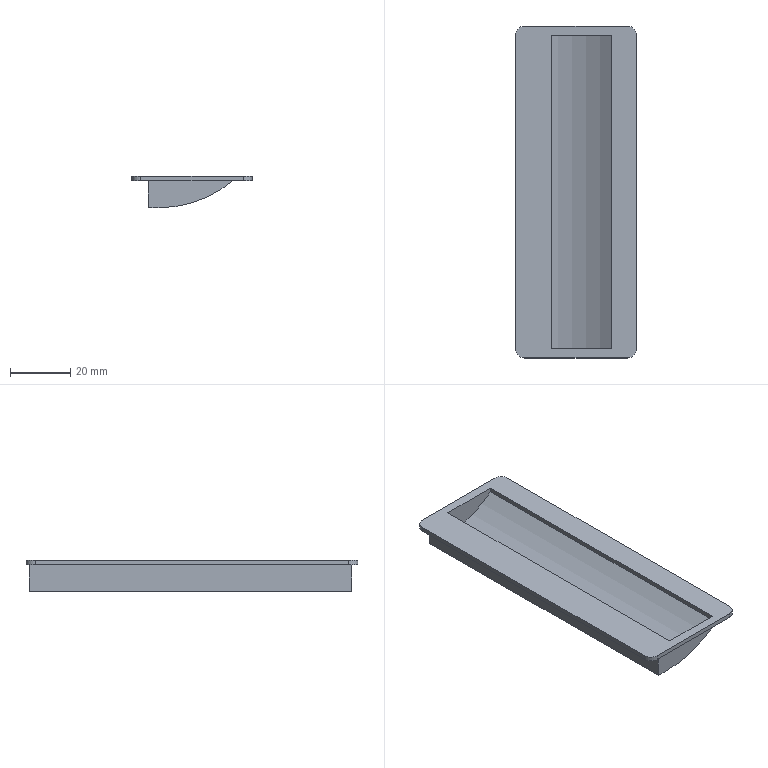Part | SolidWorks | features ICE 3, Extrusion 1, Fillet 1, MirrorPattern 1 | 1 solid | 23 faces | box 40 x 110 x 10.429 mm | volume 7857 mm3 | plane 15 | cylinder 8 | commonest cylinder face diameters 6 x4 73.801 x2 75.801 x2
STEP:
#1=CARTESIAN_POINT('',(-10.931,54.,-8.929));
#2=VERTEX_POINT('',#1);
#3=CARTESIAN_POINT('',(-14.495,54.,-8.761));
#4=VERTEX_POINT('',#3);
#5=CARTESIAN_POINT('',(-10.931,54.,28.971));
#6=DIRECTION('',(0.,1.,0.));
#7=DIRECTION('',(0.,0.,1.));
#8=AXIS2_PLACEMENT_3D('',#5,#6,#7);
#9=CIRCLE('',#8,37.9);
#10=EDGE_CURVE('',#2,#4,#9,.T.);
#11=ORIENTED_EDGE('',*,*,#10,.F.);
#12=CARTESIAN_POINT('',(-10.931,-53.,-8.929));
#13=VERTEX_POINT('',#12);
#14=CARTESIAN_POINT('',(-10.931,52.5,-8.929));
#15=DIRECTION('',(0.,-1.,0.));
#16=VECTOR('',#15,1000.);
#17=LINE('',#14,#16);
#18=EDGE_CURVE('',#2,#13,#17,.T.);
#19=ORIENTED_EDGE('',*,*,#18,.T.);
#20=CARTESIAN_POINT('',(-14.495,-53.,-8.761));
#21=VERTEX_POINT('',#20);
#22=CARTESIAN_POINT('',(-10.931,-53.,28.971));
#23=DIRECTION('',(0.,1.,0.));
#24=DIRECTION('',(0.,0.,1.));
#25=AXIS2_PLACEMENT_3D('',#22,#23,#24);
#26=CIRCLE('',#25,37.9);
#27=EDGE_CURVE('',#13,#21,#26,.T.);
#28=ORIENTED_EDGE('',*,*,#27,.T.);
#29=CARTESIAN_POINT('',(-14.495,52.5,-8.761));
#30=DIRECTION('',(0.,-1.,0.));
#31=VECTOR('',#30,1000.);
#32=LINE('',#29,#31);
#33=EDGE_CURVE('',#4,#21,#32,.T.);
#34=ORIENTED_EDGE('',*,*,#33,.F.);
#35=EDGE_LOOP('',(#11,#19,#28,#34));
#36=FACE_OUTER_BOUND('',#35,.T.);
#37=CARTESIAN_POINT('',(-10.931,52.5,28.971));
#38=DIRECTION('',(0.,-1.,0.));
#39=DIRECTION('',(0.,0.,-1.));
#40=AXIS2_PLACEMENT_3D('',#37,#38,#39);
#41=CYLINDRICAL_SURFACE('',#40,37.9);
#42=ADVANCED_FACE('',(#36),#41,.T.);
#43=CARTESIAN_POINT('',(-10.931,52.,-7.929));
#44=VERTEX_POINT('',#43);
#45=CARTESIAN_POINT('',(11.923,52.,0.));
#46=VERTEX_POINT('',#45);
#47=CARTESIAN_POINT('',(-10.931,52.,28.971));
#48=DIRECTION('',(0.,-1.,0.));
#49=DIRECTION('',(0.,0.,1.));
#50=AXIS2_PLACEMENT_3D('',#47,#48,#49);
#51=CIRCLE('',#50,36.9);
#52=EDGE_CURVE('',#44,#46,#51,.T.);
#53=ORIENTED_EDGE('',*,*,#52,.F.);
#54=CARTESIAN_POINT('',(-10.931,-52.,-7.929));
#55=VERTEX_POINT('',#54);
#56=CARTESIAN_POINT('',(-10.931,52.5,-7.929));
#57=DIRECTION('',(0.,-1.,0.));
#58=VECTOR('',#57,1000.);
#59=LINE('',#56,#58);
#60=EDGE_CURVE('',#44,#55,#59,.T.);
#61=ORIENTED_EDGE('',*,*,#60,.T.);
#62=CARTESIAN_POINT('',(11.923,-52.,0.));
#63=VERTEX_POINT('',#62);
#64=CARTESIAN_POINT('',(-10.931,-52.,28.971));
#65=DIRECTION('',(0.,1.,0.));
#66=DIRECTION('',(0.,0.,-1.));
#67=AXIS2_PLACEMENT_3D('',#64,#65,#66);
#68=CIRCLE('',#67,36.9);
#69=EDGE_CURVE('',#63,#55,#68,.T.);
#70=ORIENTED_EDGE('',*,*,#69,.F.);
#71=CARTESIAN_POINT('',(11.923,52.5,0.));
#72=DIRECTION('',(0.,-1.,0.));
#73=VECTOR('',#72,1000.);
#74=LINE('',#71,#73);
#75=EDGE_CURVE('',#46,#63,#74,.T.);
#76=ORIENTED_EDGE('',*,*,#75,.F.);
#77=EDGE_LOOP('',(#53,#61,#70,#76));
#78=FACE_OUTER_BOUND('',#77,.T.);
#79=CARTESIAN_POINT('',(-10.931,52.5,28.971));
#80=DIRECTION('',(0.,-1.,0.));
#81=DIRECTION('',(0.,0.,-1.));
#82=AXIS2_PLACEMENT_3D('',#79,#80,#81);
#83=CYLINDRICAL_SURFACE('',#82,36.9);
#84=ADVANCED_FACE('',(#78),#83,.F.);
#85=ORIENTED_EDGE('',*,*,#69,.T.);
#86=CARTESIAN_POINT('',(-13.495,-52.,-7.84));
#87=VERTEX_POINT('',#86);
#88=CARTESIAN_POINT('',(-10.931,-52.,28.971));
#89=DIRECTION('',(0.,1.,0.));
#90=DIRECTION('',(0.,0.,-1.));
#91=AXIS2_PLACEMENT_3D('',#88,#89,#90);
#92=CIRCLE('',#91,36.9);
#93=EDGE_CURVE('',#55,#87,#92,.T.);
#94=ORIENTED_EDGE('',*,*,#93,.T.);
#95=CARTESIAN_POINT('',(-13.495,-52.,0.));
#96=VERTEX_POINT('',#95);
#97=CARTESIAN_POINT('',(-13.495,-52.,0.));
#98=DIRECTION('',(0.,0.,1.));
#99=VECTOR('',#98,1000.);
#100=LINE('',#97,#99);
#101=EDGE_CURVE('',#87,#96,#100,.T.);
#102=ORIENTED_EDGE('',*,*,#101,.T.);
#103=CARTESIAN_POINT('',(-8.077,-52.,0.));
#104=VERTEX_POINT('',#103);
#105=CARTESIAN_POINT('',(-14.495,-52.,0.));
#106=DIRECTION('',(1.,0.,0.));
#107=VECTOR('',#106,1000.);
#108=LINE('',#105,#107);
#109=EDGE_CURVE('',#96,#104,#108,.T.);
#110=ORIENTED_EDGE('',*,*,#109,.T.);
#111=CARTESIAN_POINT('',(-8.077,-52.,1.5));
#112=VERTEX_POINT('',#111);
#113=CARTESIAN_POINT('',(-8.077,-52.,0.));
#114=DIRECTION('',(0.,0.,1.));
#115=VECTOR('',#114,1000.);
#116=LINE('',#113,#115);
#117=EDGE_CURVE('',#104,#112,#116,.T.);
#118=ORIENTED_EDGE('',*,*,#117,.T.);
#119=CARTESIAN_POINT('',(11.923,-52.,1.5));
#120=VERTEX_POINT('',#119);
#121=CARTESIAN_POINT('',(-8.077,-52.,1.5));
#122=DIRECTION('',(1.,0.,0.));
#123=VECTOR('',#122,1000.);
#124=LINE('',#121,#123);
#125=EDGE_CURVE('',#112,#120,#124,.T.);
#126=ORIENTED_EDGE('',*,*,#125,.T.);
#127=CARTESIAN_POINT('',(11.923,-52.,0.));
#128=DIRECTION('',(0.,0.,1.));
#129=VECTOR('',#128,1000.);
#130=LINE('',#127,#129);
#131=EDGE_CURVE('',#63,#120,#130,.T.);
#132=ORIENTED_EDGE('',*,*,#131,.F.);
#133=EDGE_LOOP('',(#85,#94,#102,#110,#118,#126,#132));
#134=FACE_OUTER_BOUND('',#133,.T.);
#135=CARTESIAN_POINT('',(-10.931,-52.,28.971));
#136=DIRECTION('',(0.,-1.,0.));
#137=DIRECTION('',(0.,0.,1.));
#138=AXIS2_PLACEMENT_3D('',#135,#136,#137);
#139=PLANE('',#138);
#140=ADVANCED_FACE('',(#134),#139,.F.);
#141=CARTESIAN_POINT('',(-13.495,52.,0.));
#142=VERTEX_POINT('',#141);
#143=CARTESIAN_POINT('',(-8.077,52.,0.));
#144=VERTEX_POINT('',#143);
#145=CARTESIAN_POINT('',(11.923,52.,0.));
#146=DIRECTION('',(1.,0.,0.));
#147=VECTOR('',#146,1000.);
#148=LINE('',#145,#147);
#149=EDGE_CURVE('',#142,#144,#148,.T.);
#150=ORIENTED_EDGE('',*,*,#149,.F.);
#151=CARTESIAN_POINT('',(-13.495,52.,-7.84));
#152=VERTEX_POINT('',#151);
#153=CARTESIAN_POINT('',(-13.495,52.,0.));
#154=DIRECTION('',(0.,0.,-1.));
#155=VECTOR('',#154,1000.);
#156=LINE('',#153,#155);
#157=EDGE_CURVE('',#142,#152,#156,.T.);
#158=ORIENTED_EDGE('',*,*,#157,.T.);
#159=CARTESIAN_POINT('',(-10.931,52.,28.971));
#160=DIRECTION('',(0.,-1.,0.));
#161=DIRECTION('',(0.,0.,1.));
#162=AXIS2_PLACEMENT_3D('',#159,#160,#161);
#163=CIRCLE('',#162,36.9);
#164=EDGE_CURVE('',#152,#44,#163,.T.);
#165=ORIENTED_EDGE('',*,*,#164,.T.);
#166=ORIENTED_EDGE('',*,*,#52,.T.);
#167=CARTESIAN_POINT('',(11.923,52.,1.5));
#168=VERTEX_POINT('',#167);
#169=CARTESIAN_POINT('',(11.923,52.,0.));
#170=DIRECTION('',(0.,0.,1.));
#171=VECTOR('',#170,1000.);
#172=LINE('',#169,#171);
#173=EDGE_CURVE('',#46,#168,#172,.T.);
#174=ORIENTED_EDGE('',*,*,#173,.T.);
#175=CARTESIAN_POINT('',(-8.077,52.,1.5));
#176=VERTEX_POINT('',#175);
#177=CARTESIAN_POINT('',(-8.077,52.,1.5));
#178=DIRECTION('',(-1.,0.,0.));
#179=VECTOR('',#178,1000.);
#180=LINE('',#177,#179);
#181=EDGE_CURVE('',#168,#176,#180,.T.);
#182=ORIENTED_EDGE('',*,*,#181,.T.);
#183=CARTESIAN_POINT('',(-8.077,52.,0.));
#184=DIRECTION('',(0.,0.,1.));
#185=VECTOR('',#184,1000.);
#186=LINE('',#183,#185);
#187=EDGE_CURVE('',#144,#176,#186,.T.);
#188=ORIENTED_EDGE('',*,*,#187,.F.);
#189=EDGE_LOOP('',(#150,#158,#165,#166,#174,#182,#188));
#190=FACE_OUTER_BOUND('',#189,.T.);
#191=CARTESIAN_POINT('',(-10.931,52.,28.971));
#192=DIRECTION('',(0.,1.,0.));
#193=DIRECTION('',(0.,0.,1.));
#194=AXIS2_PLACEMENT_3D('',#191,#192,#193);
#195=PLANE('',#194);
#196=ADVANCED_FACE('',(#190),#195,.F.);
#197=ORIENTED_EDGE('',*,*,#60,.F.);
#198=ORIENTED_EDGE('',*,*,#164,.F.);
#199=CARTESIAN_POINT('',(-13.495,52.5,-7.84));
#200=DIRECTION('',(0.,-1.,0.));
#201=VECTOR('',#200,1000.);
#202=LINE('',#199,#201);
#203=EDGE_CURVE('',#152,#87,#202,.T.);
#204=ORIENTED_EDGE('',*,*,#203,.T.);
#205=ORIENTED_EDGE('',*,*,#93,.F.);
#206=EDGE_LOOP('',(#197,#198,#204,#205));
#207=FACE_OUTER_BOUND('',#206,.T.);
#208=CARTESIAN_POINT('',(-10.931,52.5,28.971));
#209=DIRECTION('',(0.,-1.,0.));
#210=DIRECTION('',(0.,0.,-1.));
#211=AXIS2_PLACEMENT_3D('',#208,#209,#210);
#212=CYLINDRICAL_SURFACE('',#211,36.9);
#213=ADVANCED_FACE('',(#207),#212,.F.);
#214=ORIENTED_EDGE('',*,*,#101,.F.);
#215=ORIENTED_EDGE('',*,*,#203,.F.);
#216=ORIENTED_EDGE('',*,*,#157,.F.);
#217=CARTESIAN_POINT('',(-13.495,52.5,0.));
#218=DIRECTION('',(0.,-1.,0.));
#219=VECTOR('',#218,1000.);
#220=LINE('',#217,#219);
#221=EDGE_CURVE('',#142,#96,#220,.T.);
#222=ORIENTED_EDGE('',*,*,#221,.T.);
#223=EDGE_LOOP('',(#214,#215,#216,#222));
#224=FACE_OUTER_BOUND('',#223,.T.);
#225=CARTESIAN_POINT('',(-13.495,52.5,0.));
#226=DIRECTION('',(-1.,0.,0.));
#227=DIRECTION('',(0.,0.,1.));
#228=AXIS2_PLACEMENT_3D('',#225,#226,#227);
#229=PLANE('',#228);
#230=ADVANCED_FACE('',(#224),#229,.F.);
#231=CARTESIAN_POINT('',(-8.077,-52.,0.));
#232=DIRECTION('',(0.,-1.,0.));
#233=VECTOR('',#232,1000.);
#234=LINE('',#231,#233);
#235=EDGE_CURVE('',#144,#104,#234,.T.);
#236=ORIENTED_EDGE('',*,*,#235,.T.);
#237=ORIENTED_EDGE('',*,*,#109,.F.);
#238=ORIENTED_EDGE('',*,*,#221,.F.);
#239=ORIENTED_EDGE('',*,*,#149,.T.);
#240=EDGE_LOOP('',(#236,#237,#238,#239));
#241=FACE_OUTER_BOUND('',#240,.T.);
#242=CARTESIAN_POINT('',(0.,0.,0.));
#243=DIRECTION('',(0.,0.,-1.));
#244=DIRECTION('',(-1.,0.,0.));
#245=AXIS2_PLACEMENT_3D('',#242,#243,#244);
#246=PLANE('',#245);
#247=ADVANCED_FACE('',(#241),#246,.T.);
#248=CARTESIAN_POINT('',(11.923,-52.,1.5));
#249=DIRECTION('',(0.,1.,0.));
#250=VECTOR('',#249,1000.);
#251=LINE('',#248,#250);
#252=EDGE_CURVE('',#120,#168,#251,.T.);
#253=ORIENTED_EDGE('',*,*,#252,.T.);
#254=ORIENTED_EDGE('',*,*,#173,.F.);
#255=ORIENTED_EDGE('',*,*,#75,.T.);
#256=ORIENTED_EDGE('',*,*,#131,.T.);
#257=EDGE_LOOP('',(#253,#254,#255,#256));
#258=FACE_OUTER_BOUND('',#257,.T.);
#259=CARTESIAN_POINT('',(11.923,-52.,0.));
#260=DIRECTION('',(1.,0.,0.));
#261=DIRECTION('',(0.,0.,-1.));
#262=AXIS2_PLACEMENT_3D('',#259,#260,#261);
#263=PLANE('',#262);
#264=ADVANCED_FACE('',(#258),#263,.F.);
#265=CARTESIAN_POINT('',(-8.077,-52.,1.5));
#266=DIRECTION('',(0.,-1.,0.));
#267=VECTOR('',#266,1000.);
#268=LINE('',#265,#267);
#269=EDGE_CURVE('',#176,#112,#268,.T.);
#270=ORIENTED_EDGE('',*,*,#269,.T.);
#271=ORIENTED_EDGE('',*,*,#117,.F.);
#272=ORIENTED_EDGE('',*,*,#235,.F.);
#273=ORIENTED_EDGE('',*,*,#187,.T.);
#274=EDGE_LOOP('',(#270,#271,#272,#273));
#275=FACE_OUTER_BOUND('',#274,.T.);
#276=CARTESIAN_POINT('',(-8.077,-52.,0.));
#277=DIRECTION('',(-1.,0.,0.));
#278=DIRECTION('',(0.,0.,1.));
#279=AXIS2_PLACEMENT_3D('',#276,#277,#278);
#280=PLANE('',#279);
#281=ADVANCED_FACE('',(#275),#280,.F.);
#282=CARTESIAN_POINT('',(-14.495,54.,0.));
#283=VERTEX_POINT('',#282);
#284=CARTESIAN_POINT('',(13.505,54.,0.));
#285=VERTEX_POINT('',#284);
#286=CARTESIAN_POINT('',(-14.495,54.,0.));
#287=DIRECTION('',(1.,0.,0.));
#288=VECTOR('',#287,1000.);
#289=LINE('',#286,#288);
#290=EDGE_CURVE('',#283,#285,#289,.T.);
#291=ORIENTED_EDGE('',*,*,#290,.F.);
#292=CARTESIAN_POINT('',(-14.495,-53.,0.));
#293=VERTEX_POINT('',#292);
#294=CARTESIAN_POINT('',(-14.495,52.5,0.));
#295=DIRECTION('',(0.,-1.,0.));
#296=VECTOR('',#295,1000.);
#297=LINE('',#294,#296);
#298=EDGE_CURVE('',#283,#293,#297,.T.);
#299=ORIENTED_EDGE('',*,*,#298,.T.);
#300=CARTESIAN_POINT('',(13.505,-53.,0.));
#301=VERTEX_POINT('',#300);
#302=CARTESIAN_POINT('',(11.923,-53.,0.));
#303=DIRECTION('',(1.,0.,0.));
#304=VECTOR('',#303,1000.);
#305=LINE('',#302,#304);
#306=EDGE_CURVE('',#293,#301,#305,.T.);
#307=ORIENTED_EDGE('',*,*,#306,.T.);
#308=CARTESIAN_POINT('',(13.505,52.5,0.));
#309=DIRECTION('',(0.,-1.,0.));
#310=VECTOR('',#309,1000.);
#311=LINE('',#308,#310);
#312=EDGE_CURVE('',#285,#301,#311,.T.);
#313=ORIENTED_EDGE('',*,*,#312,.F.);
#314=EDGE_LOOP('',(#291,#299,#307,#313));
#315=FACE_BOUND('',#314,.T.);
#316=CARTESIAN_POINT('',(20.,-52.,0.));
#317=VERTEX_POINT('',#316);
#318=CARTESIAN_POINT('',(20.,52.,0.));
#319=VERTEX_POINT('',#318);
#320=CARTESIAN_POINT('',(20.,-55.,0.));
#321=DIRECTION('',(0.,1.,0.));
#322=VECTOR('',#321,1000.);
#323=LINE('',#320,#322);
#324=EDGE_CURVE('',#317,#319,#323,.T.);
#325=ORIENTED_EDGE('',*,*,#324,.F.);
#326=CARTESIAN_POINT('',(17.,-55.,0.));
#327=VERTEX_POINT('',#326);
#328=CARTESIAN_POINT('',(17.,-52.,0.));
#329=DIRECTION('',(0.,0.,-1.));
#330=DIRECTION('',(-1.,0.,0.));
#331=AXIS2_PLACEMENT_3D('',#328,#329,#330);
#332=CIRCLE('',#331,3.);
#333=EDGE_CURVE('',#317,#327,#332,.T.);
#334=ORIENTED_EDGE('',*,*,#333,.T.);
#335=CARTESIAN_POINT('',(-17.,-55.,0.));
#336=VERTEX_POINT('',#335);
#337=CARTESIAN_POINT('',(-20.,-55.,0.));
#338=DIRECTION('',(1.,0.,0.));
#339=VECTOR('',#338,1000.);
#340=LINE('',#337,#339);
#341=EDGE_CURVE('',#336,#327,#340,.T.);
#342=ORIENTED_EDGE('',*,*,#341,.F.);
#343=CARTESIAN_POINT('',(-20.,-52.,0.));
#344=VERTEX_POINT('',#343);
#345=CARTESIAN_POINT('',(-17.,-52.,0.));
#346=DIRECTION('',(0.,0.,-1.));
#347=DIRECTION('',(-1.,0.,0.));
#348=AXIS2_PLACEMENT_3D('',#345,#346,#347);
#349=CIRCLE('',#348,3.);
#350=EDGE_CURVE('',#336,#344,#349,.T.);
#351=ORIENTED_EDGE('',*,*,#350,.T.);
#352=CARTESIAN_POINT('',(-20.,52.,0.));
#353=VERTEX_POINT('',#352);
#354=CARTESIAN_POINT('',(-20.,-55.,0.));
#355=DIRECTION('',(0.,-1.,0.));
#356=VECTOR('',#355,1000.);
#357=LINE('',#354,#356);
#358=EDGE_CURVE('',#353,#344,#357,.T.);
#359=ORIENTED_EDGE('',*,*,#358,.F.);
#360=CARTESIAN_POINT('',(-17.,55.,0.));
#361=VERTEX_POINT('',#360);
#362=CARTESIAN_POINT('',(-17.,52.,0.));
#363=DIRECTION('',(0.,0.,-1.));
#364=DIRECTION('',(-1.,0.,0.));
#365=AXIS2_PLACEMENT_3D('',#362,#363,#364);
#366=CIRCLE('',#365,3.);
#367=EDGE_CURVE('',#353,#361,#366,.T.);
#368=ORIENTED_EDGE('',*,*,#367,.T.);
#369=CARTESIAN_POINT('',(17.,55.,0.));
#370=VERTEX_POINT('',#369);
#371=CARTESIAN_POINT('',(-20.,55.,0.));
#372=DIRECTION('',(-1.,0.,0.));
#373=VECTOR('',#372,1000.);
#374=LINE('',#371,#373);
#375=EDGE_CURVE('',#370,#361,#374,.T.);
#376=ORIENTED_EDGE('',*,*,#375,.F.);
#377=CARTESIAN_POINT('',(17.,52.,0.));
#378=DIRECTION('',(0.,0.,-1.));
#379=DIRECTION('',(-1.,0.,0.));
#380=AXIS2_PLACEMENT_3D('',#377,#378,#379);
#381=CIRCLE('',#380,3.);
#382=EDGE_CURVE('',#370,#319,#381,.T.);
#383=ORIENTED_EDGE('',*,*,#382,.T.);
#384=EDGE_LOOP('',(#325,#334,#342,#351,#359,#368,#376,#383));
#385=FACE_OUTER_BOUND('',#384,.T.);
#386=CARTESIAN_POINT('',(0.,0.,0.));
#387=DIRECTION('',(0.,0.,-1.));
#388=DIRECTION('',(-1.,0.,0.));
#389=AXIS2_PLACEMENT_3D('',#386,#387,#388);
#390=PLANE('',#389);
#391=ADVANCED_FACE('',(#315,#385),#390,.T.);
#392=CARTESIAN_POINT('',(20.,-52.,1.5));
#393=VERTEX_POINT('',#392);
#394=CARTESIAN_POINT('',(20.,52.,1.5));
#395=VERTEX_POINT('',#394);
#396=CARTESIAN_POINT('',(20.,-55.,1.5));
#397=DIRECTION('',(0.,1.,0.));
#398=VECTOR('',#397,1000.);
#399=LINE('',#396,#398);
#400=EDGE_CURVE('',#393,#395,#399,.T.);
#401=ORIENTED_EDGE('',*,*,#400,.F.);
#402=CARTESIAN_POINT('',(20.,-52.,1.5));
#403=DIRECTION('',(0.,0.,-1.));
#404=VECTOR('',#403,1000.);
#405=LINE('',#402,#404);
#406=EDGE_CURVE('',#393,#317,#405,.T.);
#407=ORIENTED_EDGE('',*,*,#406,.T.);
#408=ORIENTED_EDGE('',*,*,#324,.T.);
#409=CARTESIAN_POINT('',(20.,52.,1.5));
#410=DIRECTION('',(0.,0.,1.));
#411=VECTOR('',#410,1000.);
#412=LINE('',#409,#411);
#413=EDGE_CURVE('',#319,#395,#412,.T.);
#414=ORIENTED_EDGE('',*,*,#413,.T.);
#415=EDGE_LOOP('',(#401,#407,#408,#414));
#416=FACE_OUTER_BOUND('',#415,.T.);
#417=CARTESIAN_POINT('',(20.,-55.,1.5));
#418=DIRECTION('',(-1.,0.,0.));
#419=DIRECTION('',(0.,0.,1.));
#420=AXIS2_PLACEMENT_3D('',#417,#418,#419);
#421=PLANE('',#420);
#422=ADVANCED_FACE('',(#416),#421,.F.);
#423=ORIENTED_EDGE('',*,*,#375,.T.);
#424=CARTESIAN_POINT('',(-17.,55.,1.5));
#425=VERTEX_POINT('',#424);
#426=CARTESIAN_POINT('',(-17.,55.,1.5));
#427=DIRECTION('',(0.,0.,1.));
#428=VECTOR('',#427,1000.);
#429=LINE('',#426,#428);
#430=EDGE_CURVE('',#361,#425,#429,.T.);
#431=ORIENTED_EDGE('',*,*,#430,.T.);
#432=CARTESIAN_POINT('',(17.,55.,1.5));
#433=VERTEX_POINT('',#432);
#434=CARTESIAN_POINT('',(-20.,55.,1.5));
#435=DIRECTION('',(-1.,0.,0.));
#436=VECTOR('',#435,1000.);
#437=LINE('',#434,#436);
#438=EDGE_CURVE('',#433,#425,#437,.T.);
#439=ORIENTED_EDGE('',*,*,#438,.F.);
#440=CARTESIAN_POINT('',(17.,55.,1.5));
#441=DIRECTION('',(0.,0.,-1.));
#442=VECTOR('',#441,1000.);
#443=LINE('',#440,#442);
#444=EDGE_CURVE('',#433,#370,#443,.T.);
#445=ORIENTED_EDGE('',*,*,#444,.T.);
#446=EDGE_LOOP('',(#423,#431,#439,#445));
#447=FACE_OUTER_BOUND('',#446,.T.);
#448=CARTESIAN_POINT('',(-20.,55.,1.5));
#449=DIRECTION('',(0.,-1.,0.));
#450=DIRECTION('',(0.,0.,-1.));
#451=AXIS2_PLACEMENT_3D('',#448,#449,#450);
#452=PLANE('',#451);
#453=ADVANCED_FACE('',(#447),#452,.F.);
#454=ORIENTED_EDGE('',*,*,#358,.T.);
#455=CARTESIAN_POINT('',(-20.,-52.,1.5));
#456=VERTEX_POINT('',#455);
#457=CARTESIAN_POINT('',(-20.,-52.,1.5));
#458=DIRECTION('',(0.,0.,1.));
#459=VECTOR('',#458,1000.);
#460=LINE('',#457,#459);
#461=EDGE_CURVE('',#344,#456,#460,.T.);
#462=ORIENTED_EDGE('',*,*,#461,.T.);
#463=CARTESIAN_POINT('',(-20.,52.,1.5));
#464=VERTEX_POINT('',#463);
#465=CARTESIAN_POINT('',(-20.,-55.,1.5));
#466=DIRECTION('',(0.,-1.,0.));
#467=VECTOR('',#466,1000.);
#468=LINE('',#465,#467);
#469=EDGE_CURVE('',#464,#456,#468,.T.);
#470=ORIENTED_EDGE('',*,*,#469,.F.);
#471=CARTESIAN_POINT('',(-20.,52.,1.5));
#472=DIRECTION('',(0.,0.,-1.));
#473=VECTOR('',#472,1000.);
#474=LINE('',#471,#473);
#475=EDGE_CURVE('',#464,#353,#474,.T.);
#476=ORIENTED_EDGE('',*,*,#475,.T.);
#477=EDGE_LOOP('',(#454,#462,#470,#476));
#478=FACE_OUTER_BOUND('',#477,.T.);
#479=CARTESIAN_POINT('',(-20.,-55.,1.5));
#480=DIRECTION('',(1.,0.,0.));
#481=DIRECTION('',(0.,0.,-1.));
#482=AXIS2_PLACEMENT_3D('',#479,#480,#481);
#483=PLANE('',#482);
#484=ADVANCED_FACE('',(#478),#483,.F.);
#485=ORIENTED_EDGE('',*,*,#341,.T.);
#486=CARTESIAN_POINT('',(17.,-55.,1.5));
#487=VERTEX_POINT('',#486);
#488=CARTESIAN_POINT('',(17.,-55.,1.5));
#489=DIRECTION('',(0.,0.,1.));
#490=VECTOR('',#489,1000.);
#491=LINE('',#488,#490);
#492=EDGE_CURVE('',#327,#487,#491,.T.);
#493=ORIENTED_EDGE('',*,*,#492,.T.);
#494=CARTESIAN_POINT('',(-17.,-55.,1.5));
#495=VERTEX_POINT('',#494);
#496=CARTESIAN_POINT('',(-20.,-55.,1.5));
#497=DIRECTION('',(1.,0.,0.));
#498=VECTOR('',#497,1000.);
#499=LINE('',#496,#498);
#500=EDGE_CURVE('',#495,#487,#499,.T.);
#501=ORIENTED_EDGE('',*,*,#500,.F.);
#502=CARTESIAN_POINT('',(-17.,-55.,1.5));
#503=DIRECTION('',(0.,0.,-1.));
#504=VECTOR('',#503,1000.);
#505=LINE('',#502,#504);
#506=EDGE_CURVE('',#495,#336,#505,.T.);
#507=ORIENTED_EDGE('',*,*,#506,.T.);
#508=EDGE_LOOP('',(#485,#493,#501,#507));
#509=FACE_OUTER_BOUND('',#508,.T.);
#510=CARTESIAN_POINT('',(-20.,-55.,1.5));
#511=DIRECTION('',(0.,1.,0.));
#512=DIRECTION('',(0.,0.,1.));
#513=AXIS2_PLACEMENT_3D('',#510,#511,#512);
#514=PLANE('',#513);
#515=ADVANCED_FACE('',(#509),#514,.F.);
#516=ORIENTED_EDGE('',*,*,#181,.F.);
#517=ORIENTED_EDGE('',*,*,#252,.F.);
#518=ORIENTED_EDGE('',*,*,#125,.F.);
#519=ORIENTED_EDGE('',*,*,#269,.F.);
#520=EDGE_LOOP('',(#516,#517,#518,#519));
#521=FACE_BOUND('',#520,.T.);
#522=ORIENTED_EDGE('',*,*,#500,.T.);
#523=CARTESIAN_POINT('',(17.,-52.,1.5));
#524=DIRECTION('',(0.,0.,1.));
#525=DIRECTION('',(-1.,0.,0.));
#526=AXIS2_PLACEMENT_3D('',#523,#524,#525);
#527=CIRCLE('',#526,3.);
#528=EDGE_CURVE('',#487,#393,#527,.T.);
#529=ORIENTED_EDGE('',*,*,#528,.T.);
#530=ORIENTED_EDGE('',*,*,#400,.T.);
#531=CARTESIAN_POINT('',(17.,52.,1.5));
#532=DIRECTION('',(0.,0.,1.));
#533=DIRECTION('',(-1.,0.,0.));
#534=AXIS2_PLACEMENT_3D('',#531,#532,#533);
#535=CIRCLE('',#534,3.);
#536=EDGE_CURVE('',#395,#433,#535,.T.);
#537=ORIENTED_EDGE('',*,*,#536,.T.);
#538=ORIENTED_EDGE('',*,*,#438,.T.);
#539=CARTESIAN_POINT('',(-17.,52.,1.5));
#540=DIRECTION('',(0.,0.,1.));
#541=DIRECTION('',(-1.,0.,0.));
#542=AXIS2_PLACEMENT_3D('',#539,#540,#541);
#543=CIRCLE('',#542,3.);
#544=EDGE_CURVE('',#425,#464,#543,.T.);
#545=ORIENTED_EDGE('',*,*,#544,.T.);
#546=ORIENTED_EDGE('',*,*,#469,.T.);
#547=CARTESIAN_POINT('',(-17.,-52.,1.5));
#548=DIRECTION('',(0.,0.,1.));
#549=DIRECTION('',(-1.,0.,0.));
#550=AXIS2_PLACEMENT_3D('',#547,#548,#549);
#551=CIRCLE('',#550,3.);
#552=EDGE_CURVE('',#456,#495,#551,.T.);
#553=ORIENTED_EDGE('',*,*,#552,.T.);
#554=EDGE_LOOP('',(#522,#529,#530,#537,#538,#545,#546,#553));
#555=FACE_OUTER_BOUND('',#554,.T.);
#556=CARTESIAN_POINT('',(0.,0.,1.5));
#557=DIRECTION('',(0.,0.,-1.));
#558=DIRECTION('',(-1.,0.,0.));
#559=AXIS2_PLACEMENT_3D('',#556,#557,#558);
#560=PLANE('',#559);
#561=ADVANCED_FACE('',(#521,#555),#560,.F.);
#562=ORIENTED_EDGE('',*,*,#18,.F.);
#563=CARTESIAN_POINT('',(-10.931,54.,28.971));
#564=DIRECTION('',(0.,1.,0.));
#565=DIRECTION('',(0.,0.,1.));
#566=AXIS2_PLACEMENT_3D('',#563,#564,#565);
#567=CIRCLE('',#566,37.9);
#568=EDGE_CURVE('',#285,#2,#567,.T.);
#569=ORIENTED_EDGE('',*,*,#568,.F.);
#570=ORIENTED_EDGE('',*,*,#312,.T.);
#571=CARTESIAN_POINT('',(-10.931,-53.,28.971));
#572=DIRECTION('',(0.,1.,0.));
#573=DIRECTION('',(0.,0.,1.));
#574=AXIS2_PLACEMENT_3D('',#571,#572,#573);
#575=CIRCLE('',#574,37.9);
#576=EDGE_CURVE('',#301,#13,#575,.T.);
#577=ORIENTED_EDGE('',*,*,#576,.T.);
#578=EDGE_LOOP('',(#562,#569,#570,#577));
#579=FACE_OUTER_BOUND('',#578,.T.);
#580=CARTESIAN_POINT('',(-10.931,52.5,28.971));
#581=DIRECTION('',(0.,-1.,0.));
#582=DIRECTION('',(0.,0.,-1.));
#583=AXIS2_PLACEMENT_3D('',#580,#581,#582);
#584=CYLINDRICAL_SURFACE('',#583,37.9);
#585=ADVANCED_FACE('',(#579),#584,.T.);
#586=CARTESIAN_POINT('',(-14.495,-53.,-8.761));
#587=DIRECTION('',(0.,0.,1.));
#588=VECTOR('',#587,1000.);
#589=LINE('',#586,#588);
#590=EDGE_CURVE('',#21,#293,#589,.T.);
#591=ORIENTED_EDGE('',*,*,#590,.T.);
#592=ORIENTED_EDGE('',*,*,#298,.F.);
#593=CARTESIAN_POINT('',(-14.495,54.,-8.761));
#594=DIRECTION('',(0.,0.,1.));
#595=VECTOR('',#594,1000.);
#596=LINE('',#593,#595);
#597=EDGE_CURVE('',#4,#283,#596,.T.);
#598=ORIENTED_EDGE('',*,*,#597,.F.);
#599=ORIENTED_EDGE('',*,*,#33,.T.);
#600=EDGE_LOOP('',(#591,#592,#598,#599));
#601=FACE_OUTER_BOUND('',#600,.T.);
#602=CARTESIAN_POINT('',(-14.495,52.5,0.));
#603=DIRECTION('',(1.,0.,0.));
#604=DIRECTION('',(0.,0.,-1.));
#605=AXIS2_PLACEMENT_3D('',#602,#603,#604);
#606=PLANE('',#605);
#607=ADVANCED_FACE('',(#601),#606,.F.);
#608=ORIENTED_EDGE('',*,*,#590,.F.);
#609=ORIENTED_EDGE('',*,*,#27,.F.);
#610=ORIENTED_EDGE('',*,*,#576,.F.);
#611=ORIENTED_EDGE('',*,*,#306,.F.);
#612=EDGE_LOOP('',(#608,#609,#610,#611));
#613=FACE_OUTER_BOUND('',#612,.T.);
#614=CARTESIAN_POINT('',(-10.931,-53.,28.971));
#615=DIRECTION('',(0.,-1.,0.));
#616=DIRECTION('',(0.,0.,1.));
#617=AXIS2_PLACEMENT_3D('',#614,#615,#616);
#618=PLANE('',#617);
#619=ADVANCED_FACE('',(#613),#618,.T.);
#620=ORIENTED_EDGE('',*,*,#597,.T.);
#621=ORIENTED_EDGE('',*,*,#290,.T.);
#622=ORIENTED_EDGE('',*,*,#568,.T.);
#623=ORIENTED_EDGE('',*,*,#10,.T.);
#624=EDGE_LOOP('',(#620,#621,#622,#623));
#625=FACE_OUTER_BOUND('',#624,.T.);
#626=CARTESIAN_POINT('',(-10.931,54.,28.971));
#627=DIRECTION('',(0.,-1.,0.));
#628=DIRECTION('',(0.,0.,1.));
#629=AXIS2_PLACEMENT_3D('',#626,#627,#628);
#630=PLANE('',#629);
#631=ADVANCED_FACE('',(#625),#630,.F.);
#632=ORIENTED_EDGE('',*,*,#528,.F.);
#633=ORIENTED_EDGE('',*,*,#492,.F.);
#634=ORIENTED_EDGE('',*,*,#333,.F.);
#635=ORIENTED_EDGE('',*,*,#406,.F.);
#636=EDGE_LOOP('',(#632,#633,#634,#635));
#637=FACE_OUTER_BOUND('',#636,.T.);
#638=CARTESIAN_POINT('',(17.,-52.,1.5));
#639=DIRECTION('',(0.,0.,-1.));
#640=DIRECTION('',(-1.,0.,0.));
#641=AXIS2_PLACEMENT_3D('',#638,#639,#640);
#642=CYLINDRICAL_SURFACE('',#641,3.);
#643=ADVANCED_FACE('',(#637),#642,.T.);
#644=ORIENTED_EDGE('',*,*,#552,.F.);
#645=ORIENTED_EDGE('',*,*,#461,.F.);
#646=ORIENTED_EDGE('',*,*,#350,.F.);
#647=ORIENTED_EDGE('',*,*,#506,.F.);
#648=EDGE_LOOP('',(#644,#645,#646,#647));
#649=FACE_OUTER_BOUND('',#648,.T.);
#650=CARTESIAN_POINT('',(-17.,-52.,1.5));
#651=DIRECTION('',(0.,0.,-1.));
#652=DIRECTION('',(-1.,0.,0.));
#653=AXIS2_PLACEMENT_3D('',#650,#651,#652);
#654=CYLINDRICAL_SURFACE('',#653,3.);
#655=ADVANCED_FACE('',(#649),#654,.T.);
#656=ORIENTED_EDGE('',*,*,#544,.F.);
#657=ORIENTED_EDGE('',*,*,#430,.F.);
#658=ORIENTED_EDGE('',*,*,#367,.F.);
#659=ORIENTED_EDGE('',*,*,#475,.F.);
#660=EDGE_LOOP('',(#656,#657,#658,#659));
#661=FACE_OUTER_BOUND('',#660,.T.);
#662=CARTESIAN_POINT('',(-17.,52.,1.5));
#663=DIRECTION('',(0.,0.,-1.));
#664=DIRECTION('',(-1.,0.,0.));
#665=AXIS2_PLACEMENT_3D('',#662,#663,#664);
#666=CYLINDRICAL_SURFACE('',#665,3.);
#667=ADVANCED_FACE('',(#661),#666,.T.);
#668=ORIENTED_EDGE('',*,*,#536,.F.);
#669=ORIENTED_EDGE('',*,*,#413,.F.);
#670=ORIENTED_EDGE('',*,*,#382,.F.);
#671=ORIENTED_EDGE('',*,*,#444,.F.);
#672=EDGE_LOOP('',(#668,#669,#670,#671));
#673=FACE_OUTER_BOUND('',#672,.T.);
#674=CARTESIAN_POINT('',(17.,52.,1.5));
#675=DIRECTION('',(0.,0.,-1.));
#676=DIRECTION('',(-1.,0.,0.));
#677=AXIS2_PLACEMENT_3D('',#674,#675,#676);
#678=CYLINDRICAL_SURFACE('',#677,3.);
#679=ADVANCED_FACE('',(#673),#678,.T.);
#680=CLOSED_SHELL('',(#42,#84,#140,#196,#213,#230,#247,#264,#281,#391,#422,#453,#484,#515,#561,#585,#607,#619,#631,#643,#655,#667,#679));
#681=MANIFOLD_SOLID_BREP('',#680);
#682=CARTESIAN_POINT('',(0.,0.,0.));
#683=DIRECTION('',(0.,0.,1.));
#684=DIRECTION('',(1.,0.,0.));
#685=AXIS2_PLACEMENT_3D('',#682,#683,#684);
#686=(LENGTH_UNIT()NAMED_UNIT(*)SI_UNIT(.MILLI.,.METRE.));
#687=UNCERTAINTY_MEASURE_WITH_UNIT(LENGTH_MEASURE(0.00001),#686,'','');
#688=(NAMED_UNIT(*)PLANE_ANGLE_UNIT()SI_UNIT($,.RADIAN.));
#689=(NAMED_UNIT(*)SI_UNIT($,.STERADIAN.)SOLID_ANGLE_UNIT());
#690=(GEOMETRIC_REPRESENTATION_CONTEXT(3)GLOBAL_UNCERTAINTY_ASSIGNED_CONTEXT((#687))GLOBAL_UNIT_ASSIGNED_CONTEXT((#686,#688,#689))REPRESENTATION_CONTEXT('',''));
#691=ADVANCED_BREP_SHAPE_REPRESENTATION('',(#681,#685),#690);